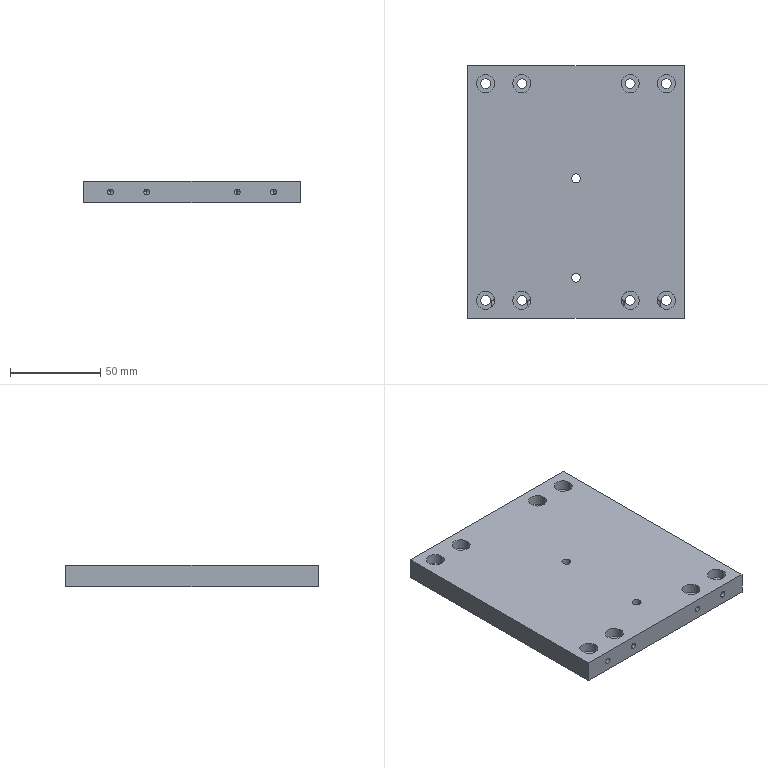Part | SolidWorks | features HoleWzd 3, 3DProfileFeature 2, Extrusion 1, ICE 1, MirrorPattern 1 | 1 solid | 76 faces | box 120 x 140 x 12 mm | volume 195775 mm3 | cylinder 52 | plane 16 | cone 8 | commonest cylinder face diameters 5.5 x16 10 x16 3.3 x12 5 x8